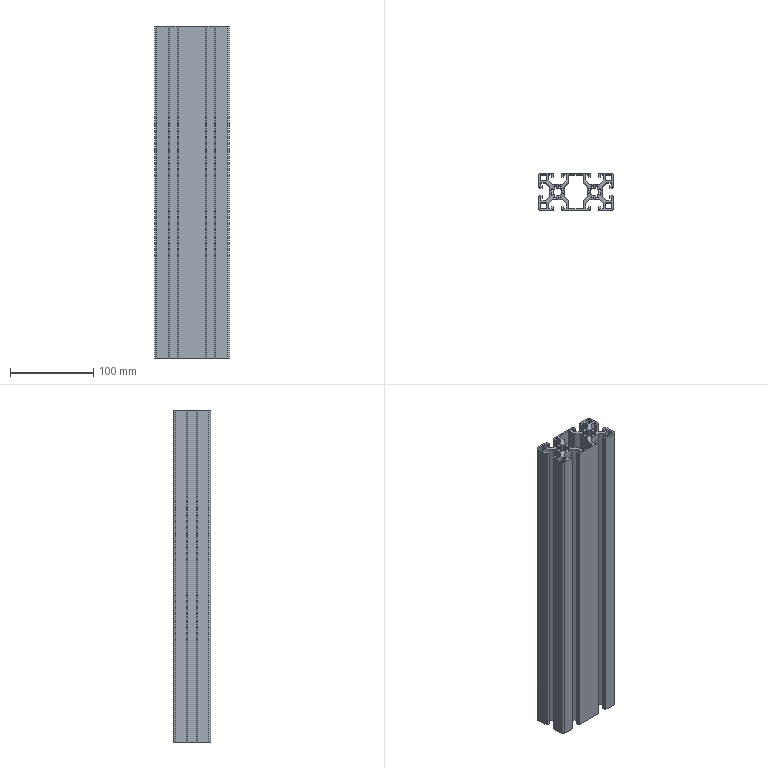Part | STEP file | OB4590-L1 | 1 solid | 256 faces | box 90 x 45 x 400 mm | volume 511223 mm3 | plane 174 | cylinder 82 | commonest cylinder face diameters 1 x24 2 x20 10.2 x18 16 x16 5 x4